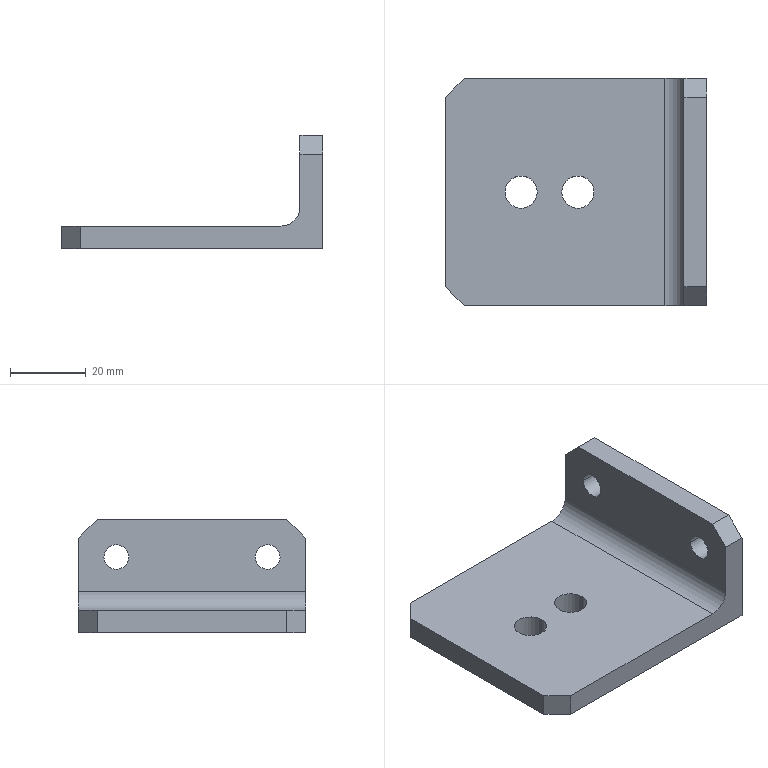Part | SolidWorks | features ICE 3, Chamfer 1, Extrusion 1, Fillet 1 | 1 solid | 21 faces | box 69 x 60 x 30 mm | volume 32423 mm3 | plane 12 | cylinder 9 | commonest cylinder face diameters 6.5 x4 8.5 x4 10 x1
STEP:
#1=CARTESIAN_POINT('',(34.5,23.25,17.));
#2=VERTEX_POINT('',#1);
#3=CARTESIAN_POINT('',(34.5,16.75,17.));
#4=VERTEX_POINT('',#3);
#5=CARTESIAN_POINT('',(34.5,20.,17.));
#6=DIRECTION('',(-1.,0.,0.));
#7=DIRECTION('',(0.,-1.,0.));
#8=AXIS2_PLACEMENT_3D('',#5,#6,#7);
#9=CIRCLE('',#8,3.25);
#10=EDGE_CURVE('',#2,#4,#9,.T.);
#11=ORIENTED_EDGE('',*,*,#10,.F.);
#12=CARTESIAN_POINT('',(28.5,23.25,17.));
#13=VERTEX_POINT('',#12);
#14=CARTESIAN_POINT('',(34.5,23.25,17.));
#15=DIRECTION('',(-1.,0.,0.));
#16=VECTOR('',#15,1000.);
#17=LINE('',#14,#16);
#18=EDGE_CURVE('',#2,#13,#17,.T.);
#19=ORIENTED_EDGE('',*,*,#18,.T.);
#20=CARTESIAN_POINT('',(28.5,16.75,17.));
#21=VERTEX_POINT('',#20);
#22=CARTESIAN_POINT('',(28.5,20.,17.));
#23=DIRECTION('',(-1.,0.,0.));
#24=DIRECTION('',(0.,-1.,0.));
#25=AXIS2_PLACEMENT_3D('',#22,#23,#24);
#26=CIRCLE('',#25,3.25);
#27=EDGE_CURVE('',#13,#21,#26,.T.);
#28=ORIENTED_EDGE('',*,*,#27,.T.);
#29=CARTESIAN_POINT('',(34.5,16.75,17.));
#30=DIRECTION('',(-1.,0.,0.));
#31=VECTOR('',#30,1000.);
#32=LINE('',#29,#31);
#33=EDGE_CURVE('',#4,#21,#32,.T.);
#34=ORIENTED_EDGE('',*,*,#33,.F.);
#35=EDGE_LOOP('',(#11,#19,#28,#34));
#36=FACE_OUTER_BOUND('',#35,.T.);
#37=CARTESIAN_POINT('',(34.5,20.,17.));
#38=DIRECTION('',(-1.,0.,0.));
#39=DIRECTION('',(0.,-1.,0.));
#40=AXIS2_PLACEMENT_3D('',#37,#38,#39);
#41=CYLINDRICAL_SURFACE('',#40,3.25);
#42=ADVANCED_FACE('',(#36),#41,.F.);
#43=CARTESIAN_POINT('',(34.5,-16.75,17.));
#44=VERTEX_POINT('',#43);
#45=CARTESIAN_POINT('',(34.5,-23.25,17.));
#46=VERTEX_POINT('',#45);
#47=CARTESIAN_POINT('',(34.5,-20.,17.));
#48=DIRECTION('',(-1.,0.,0.));
#49=DIRECTION('',(0.,-1.,0.));
#50=AXIS2_PLACEMENT_3D('',#47,#48,#49);
#51=CIRCLE('',#50,3.25);
#52=EDGE_CURVE('',#44,#46,#51,.T.);
#53=ORIENTED_EDGE('',*,*,#52,.F.);
#54=CARTESIAN_POINT('',(28.5,-16.75,17.));
#55=VERTEX_POINT('',#54);
#56=CARTESIAN_POINT('',(34.5,-16.75,17.));
#57=DIRECTION('',(-1.,0.,0.));
#58=VECTOR('',#57,1000.);
#59=LINE('',#56,#58);
#60=EDGE_CURVE('',#44,#55,#59,.T.);
#61=ORIENTED_EDGE('',*,*,#60,.T.);
#62=CARTESIAN_POINT('',(28.5,-23.25,17.));
#63=VERTEX_POINT('',#62);
#64=CARTESIAN_POINT('',(28.5,-20.,17.));
#65=DIRECTION('',(-1.,0.,0.));
#66=DIRECTION('',(0.,-1.,0.));
#67=AXIS2_PLACEMENT_3D('',#64,#65,#66);
#68=CIRCLE('',#67,3.25);
#69=EDGE_CURVE('',#55,#63,#68,.T.);
#70=ORIENTED_EDGE('',*,*,#69,.T.);
#71=CARTESIAN_POINT('',(34.5,-23.25,17.));
#72=DIRECTION('',(-1.,0.,0.));
#73=VECTOR('',#72,1000.);
#74=LINE('',#71,#73);
#75=EDGE_CURVE('',#46,#63,#74,.T.);
#76=ORIENTED_EDGE('',*,*,#75,.F.);
#77=EDGE_LOOP('',(#53,#61,#70,#76));
#78=FACE_OUTER_BOUND('',#77,.T.);
#79=CARTESIAN_POINT('',(34.5,-20.,17.));
#80=DIRECTION('',(-1.,0.,0.));
#81=DIRECTION('',(0.,-1.,0.));
#82=AXIS2_PLACEMENT_3D('',#79,#80,#81);
#83=CYLINDRICAL_SURFACE('',#82,3.25);
#84=ADVANCED_FACE('',(#78),#83,.F.);
#85=CARTESIAN_POINT('',(-18.75,0.,-3.));
#86=VERTEX_POINT('',#85);
#87=CARTESIAN_POINT('',(-10.25,0.,-3.));
#88=VERTEX_POINT('',#87);
#89=CARTESIAN_POINT('',(-14.5,0.,-3.));
#90=DIRECTION('',(0.,0.,1.));
#91=DIRECTION('',(1.,0.,0.));
#92=AXIS2_PLACEMENT_3D('',#89,#90,#91);
#93=CIRCLE('',#92,4.25);
#94=EDGE_CURVE('',#86,#88,#93,.T.);
#95=ORIENTED_EDGE('',*,*,#94,.F.);
#96=CARTESIAN_POINT('',(-18.75,0.,3.));
#97=VERTEX_POINT('',#96);
#98=CARTESIAN_POINT('',(-18.75,0.,-3.));
#99=DIRECTION('',(0.,0.,1.));
#100=VECTOR('',#99,1000.);
#101=LINE('',#98,#100);
#102=EDGE_CURVE('',#86,#97,#101,.T.);
#103=ORIENTED_EDGE('',*,*,#102,.T.);
#104=CARTESIAN_POINT('',(-10.25,0.,3.));
#105=VERTEX_POINT('',#104);
#106=CARTESIAN_POINT('',(-14.5,0.,3.));
#107=DIRECTION('',(0.,0.,1.));
#108=DIRECTION('',(1.,0.,0.));
#109=AXIS2_PLACEMENT_3D('',#106,#107,#108);
#110=CIRCLE('',#109,4.25);
#111=EDGE_CURVE('',#97,#105,#110,.T.);
#112=ORIENTED_EDGE('',*,*,#111,.T.);
#113=CARTESIAN_POINT('',(-10.25,0.,-3.));
#114=DIRECTION('',(0.,0.,1.));
#115=VECTOR('',#114,1000.);
#116=LINE('',#113,#115);
#117=EDGE_CURVE('',#88,#105,#116,.T.);
#118=ORIENTED_EDGE('',*,*,#117,.F.);
#119=EDGE_LOOP('',(#95,#103,#112,#118));
#120=FACE_OUTER_BOUND('',#119,.T.);
#121=CARTESIAN_POINT('',(-14.5,0.,-3.));
#122=DIRECTION('',(0.,0.,1.));
#123=DIRECTION('',(1.,0.,0.));
#124=AXIS2_PLACEMENT_3D('',#121,#122,#123);
#125=CYLINDRICAL_SURFACE('',#124,4.25);
#126=ADVANCED_FACE('',(#120),#125,.F.);
#127=CARTESIAN_POINT('',(-3.75,0.,-3.));
#128=VERTEX_POINT('',#127);
#129=CARTESIAN_POINT('',(4.75,0.,-3.));
#130=VERTEX_POINT('',#129);
#131=CARTESIAN_POINT('',(0.5,0.,-3.));
#132=DIRECTION('',(0.,0.,1.));
#133=DIRECTION('',(1.,0.,0.));
#134=AXIS2_PLACEMENT_3D('',#131,#132,#133);
#135=CIRCLE('',#134,4.25);
#136=EDGE_CURVE('',#128,#130,#135,.T.);
#137=ORIENTED_EDGE('',*,*,#136,.F.);
#138=CARTESIAN_POINT('',(-3.75,0.,3.));
#139=VERTEX_POINT('',#138);
#140=CARTESIAN_POINT('',(-3.75,0.,-3.));
#141=DIRECTION('',(0.,0.,1.));
#142=VECTOR('',#141,1000.);
#143=LINE('',#140,#142);
#144=EDGE_CURVE('',#128,#139,#143,.T.);
#145=ORIENTED_EDGE('',*,*,#144,.T.);
#146=CARTESIAN_POINT('',(4.75,0.,3.));
#147=VERTEX_POINT('',#146);
#148=CARTESIAN_POINT('',(0.5,0.,3.));
#149=DIRECTION('',(0.,0.,1.));
#150=DIRECTION('',(1.,0.,0.));
#151=AXIS2_PLACEMENT_3D('',#148,#149,#150);
#152=CIRCLE('',#151,4.25);
#153=EDGE_CURVE('',#139,#147,#152,.T.);
#154=ORIENTED_EDGE('',*,*,#153,.T.);
#155=CARTESIAN_POINT('',(4.75,0.,-3.));
#156=DIRECTION('',(0.,0.,1.));
#157=VECTOR('',#156,1000.);
#158=LINE('',#155,#157);
#159=EDGE_CURVE('',#130,#147,#158,.T.);
#160=ORIENTED_EDGE('',*,*,#159,.F.);
#161=EDGE_LOOP('',(#137,#145,#154,#160));
#162=FACE_OUTER_BOUND('',#161,.T.);
#163=CARTESIAN_POINT('',(0.5,0.,-3.));
#164=DIRECTION('',(0.,0.,1.));
#165=DIRECTION('',(1.,0.,0.));
#166=AXIS2_PLACEMENT_3D('',#163,#164,#165);
#167=CYLINDRICAL_SURFACE('',#166,4.25);
#168=ADVANCED_FACE('',(#162),#167,.F.);
#169=CARTESIAN_POINT('',(-34.5,25.,3.));
#170=VERTEX_POINT('',#169);
#171=CARTESIAN_POINT('',(-34.5,-25.,3.));
#172=VERTEX_POINT('',#171);
#173=CARTESIAN_POINT('',(-34.5,-30.,3.));
#174=DIRECTION('',(0.,-1.,0.));
#175=VECTOR('',#174,1000.);
#176=LINE('',#173,#175);
#177=EDGE_CURVE('',#170,#172,#176,.T.);
#178=ORIENTED_EDGE('',*,*,#177,.F.);
#179=CARTESIAN_POINT('',(-34.5,25.,-3.));
#180=VERTEX_POINT('',#179);
#181=CARTESIAN_POINT('',(-34.5,25.,3.));
#182=DIRECTION('',(0.,0.,-1.));
#183=VECTOR('',#182,1000.);
#184=LINE('',#181,#183);
#185=EDGE_CURVE('',#170,#180,#184,.T.);
#186=ORIENTED_EDGE('',*,*,#185,.T.);
#187=CARTESIAN_POINT('',(-34.5,-25.,-3.));
#188=VERTEX_POINT('',#187);
#189=CARTESIAN_POINT('',(-34.5,-30.,-3.));
#190=DIRECTION('',(0.,-1.,0.));
#191=VECTOR('',#190,1000.);
#192=LINE('',#189,#191);
#193=EDGE_CURVE('',#180,#188,#192,.T.);
#194=ORIENTED_EDGE('',*,*,#193,.T.);
#195=CARTESIAN_POINT('',(-34.5,-25.,3.));
#196=DIRECTION('',(0.,0.,1.));
#197=VECTOR('',#196,1000.);
#198=LINE('',#195,#197);
#199=EDGE_CURVE('',#188,#172,#198,.T.);
#200=ORIENTED_EDGE('',*,*,#199,.T.);
#201=EDGE_LOOP('',(#178,#186,#194,#200));
#202=FACE_OUTER_BOUND('',#201,.T.);
#203=CARTESIAN_POINT('',(-34.5,-30.,3.));
#204=DIRECTION('',(1.,0.,0.));
#205=DIRECTION('',(0.,0.,-1.));
#206=AXIS2_PLACEMENT_3D('',#203,#204,#205);
#207=PLANE('',#206);
#208=ADVANCED_FACE('',(#202),#207,.F.);
#209=CARTESIAN_POINT('',(-29.5,-30.,3.));
#210=VERTEX_POINT('',#209);
#211=CARTESIAN_POINT('',(23.5,-30.,3.));
#212=VERTEX_POINT('',#211);
#213=CARTESIAN_POINT('',(34.5,-30.,3.));
#214=DIRECTION('',(1.,0.,0.));
#215=VECTOR('',#214,1000.);
#216=LINE('',#213,#215);
#217=EDGE_CURVE('',#210,#212,#216,.T.);
#218=ORIENTED_EDGE('',*,*,#217,.F.);
#219=CARTESIAN_POINT('',(-29.5,-30.,-3.));
#220=VERTEX_POINT('',#219);
#221=CARTESIAN_POINT('',(-29.5,-30.,3.));
#222=DIRECTION('',(0.,0.,-1.));
#223=VECTOR('',#222,1000.);
#224=LINE('',#221,#223);
#225=EDGE_CURVE('',#210,#220,#224,.T.);
#226=ORIENTED_EDGE('',*,*,#225,.T.);
#227=CARTESIAN_POINT('',(34.5,-30.,-3.));
#228=VERTEX_POINT('',#227);
#229=CARTESIAN_POINT('',(34.5,-30.,-3.));
#230=DIRECTION('',(1.,0.,0.));
#231=VECTOR('',#230,1000.);
#232=LINE('',#229,#231);
#233=EDGE_CURVE('',#220,#228,#232,.T.);
#234=ORIENTED_EDGE('',*,*,#233,.T.);
#235=CARTESIAN_POINT('',(34.5,-30.,22.));
#236=VERTEX_POINT('',#235);
#237=CARTESIAN_POINT('',(34.5,-30.,3.));
#238=DIRECTION('',(0.,0.,-1.));
#239=VECTOR('',#238,1000.);
#240=LINE('',#237,#239);
#241=EDGE_CURVE('',#236,#228,#240,.T.);
#242=ORIENTED_EDGE('',*,*,#241,.F.);
#243=CARTESIAN_POINT('',(28.5,-30.,22.));
#244=VERTEX_POINT('',#243);
#245=CARTESIAN_POINT('',(34.5,-30.,22.));
#246=DIRECTION('',(-1.,0.,0.));
#247=VECTOR('',#246,1000.);
#248=LINE('',#245,#247);
#249=EDGE_CURVE('',#236,#244,#248,.T.);
#250=ORIENTED_EDGE('',*,*,#249,.T.);
#251=CARTESIAN_POINT('',(28.5,-30.,8.));
#252=VERTEX_POINT('',#251);
#253=CARTESIAN_POINT('',(28.5,-30.,27.));
#254=DIRECTION('',(0.,0.,-1.));
#255=VECTOR('',#254,1000.);
#256=LINE('',#253,#255);
#257=EDGE_CURVE('',#244,#252,#256,.T.);
#258=ORIENTED_EDGE('',*,*,#257,.T.);
#259=CARTESIAN_POINT('',(23.5,-30.,8.));
#260=DIRECTION('',(0.,1.,0.));
#261=DIRECTION('',(-1.,0.,0.));
#262=AXIS2_PLACEMENT_3D('',#259,#260,#261);
#263=CIRCLE('',#262,5.);
#264=EDGE_CURVE('',#252,#212,#263,.T.);
#265=ORIENTED_EDGE('',*,*,#264,.T.);
#266=EDGE_LOOP('',(#218,#226,#234,#242,#250,#258,#265));
#267=FACE_OUTER_BOUND('',#266,.T.);
#268=CARTESIAN_POINT('',(34.5,-30.,3.));
#269=DIRECTION('',(0.,1.,0.));
#270=DIRECTION('',(-1.,0.,0.));
#271=AXIS2_PLACEMENT_3D('',#268,#269,#270);
#272=PLANE('',#271);
#273=ADVANCED_FACE('',(#267),#272,.F.);
#274=CARTESIAN_POINT('',(34.5,20.,17.));
#275=DIRECTION('',(-1.,0.,0.));
#276=DIRECTION('',(0.,-1.,0.));
#277=AXIS2_PLACEMENT_3D('',#274,#275,#276);
#278=CIRCLE('',#277,3.25);
#279=EDGE_CURVE('',#4,#2,#278,.T.);
#280=ORIENTED_EDGE('',*,*,#279,.T.);
#281=ORIENTED_EDGE('',*,*,#10,.T.);
#282=EDGE_LOOP('',(#280,#281));
#283=FACE_BOUND('',#282,.T.);
#284=CARTESIAN_POINT('',(34.5,-20.,17.));
#285=DIRECTION('',(-1.,0.,0.));
#286=DIRECTION('',(0.,-1.,0.));
#287=AXIS2_PLACEMENT_3D('',#284,#285,#286);
#288=CIRCLE('',#287,3.25);
#289=EDGE_CURVE('',#46,#44,#288,.T.);
#290=ORIENTED_EDGE('',*,*,#289,.T.);
#291=ORIENTED_EDGE('',*,*,#52,.T.);
#292=EDGE_LOOP('',(#290,#291));
#293=FACE_BOUND('',#292,.T.);
#294=CARTESIAN_POINT('',(34.5,30.,22.));
#295=VERTEX_POINT('',#294);
#296=CARTESIAN_POINT('',(34.5,30.,-3.));
#297=VERTEX_POINT('',#296);
#298=CARTESIAN_POINT('',(34.5,30.,3.));
#299=DIRECTION('',(0.,0.,-1.));
#300=VECTOR('',#299,1000.);
#301=LINE('',#298,#300);
#302=EDGE_CURVE('',#295,#297,#301,.T.);
#303=ORIENTED_EDGE('',*,*,#302,.F.);
#304=CARTESIAN_POINT('',(34.5,25.,27.));
#305=VERTEX_POINT('',#304);
#306=CARTESIAN_POINT('',(34.5,25.,27.));
#307=DIRECTION('',(0.,-0.7071,0.7071));
#308=VECTOR('',#307,1000.);
#309=LINE('',#306,#308);
#310=EDGE_CURVE('',#295,#305,#309,.T.);
#311=ORIENTED_EDGE('',*,*,#310,.T.);
#312=CARTESIAN_POINT('',(34.5,-25.,27.));
#313=VERTEX_POINT('',#312);
#314=CARTESIAN_POINT('',(34.5,30.,27.));
#315=DIRECTION('',(0.,1.,0.));
#316=VECTOR('',#315,1000.);
#317=LINE('',#314,#316);
#318=EDGE_CURVE('',#313,#305,#317,.T.);
#319=ORIENTED_EDGE('',*,*,#318,.F.);
#320=CARTESIAN_POINT('',(34.5,-25.,27.));
#321=DIRECTION('',(0.,-0.7071,-0.7071));
#322=VECTOR('',#321,1000.);
#323=LINE('',#320,#322);
#324=EDGE_CURVE('',#313,#236,#323,.T.);
#325=ORIENTED_EDGE('',*,*,#324,.T.);
#326=ORIENTED_EDGE('',*,*,#241,.T.);
#327=CARTESIAN_POINT('',(34.5,-30.,-3.));
#328=DIRECTION('',(0.,1.,0.));
#329=VECTOR('',#328,1000.);
#330=LINE('',#327,#329);
#331=EDGE_CURVE('',#228,#297,#330,.T.);
#332=ORIENTED_EDGE('',*,*,#331,.T.);
#333=EDGE_LOOP('',(#303,#311,#319,#325,#326,#332));
#334=FACE_OUTER_BOUND('',#333,.T.);
#335=CARTESIAN_POINT('',(34.5,-30.,3.));
#336=DIRECTION('',(-1.,0.,0.));
#337=DIRECTION('',(0.,0.,1.));
#338=AXIS2_PLACEMENT_3D('',#335,#336,#337);
#339=PLANE('',#338);
#340=ADVANCED_FACE('',(#283,#293,#334),#339,.F.);
#341=CARTESIAN_POINT('',(-29.5,30.,-3.));
#342=VERTEX_POINT('',#341);
#343=CARTESIAN_POINT('',(34.5,30.,-3.));
#344=DIRECTION('',(-1.,0.,0.));
#345=VECTOR('',#344,1000.);
#346=LINE('',#343,#345);
#347=EDGE_CURVE('',#297,#342,#346,.T.);
#348=ORIENTED_EDGE('',*,*,#347,.T.);
#349=CARTESIAN_POINT('',(-29.5,30.,3.));
#350=VERTEX_POINT('',#349);
#351=CARTESIAN_POINT('',(-29.5,30.,3.));
#352=DIRECTION('',(0.,0.,1.));
#353=VECTOR('',#352,1000.);
#354=LINE('',#351,#353);
#355=EDGE_CURVE('',#342,#350,#354,.T.);
#356=ORIENTED_EDGE('',*,*,#355,.T.);
#357=CARTESIAN_POINT('',(23.5,30.,3.));
#358=VERTEX_POINT('',#357);
#359=CARTESIAN_POINT('',(34.5,30.,3.));
#360=DIRECTION('',(-1.,0.,0.));
#361=VECTOR('',#360,1000.);
#362=LINE('',#359,#361);
#363=EDGE_CURVE('',#358,#350,#362,.T.);
#364=ORIENTED_EDGE('',*,*,#363,.F.);
#365=CARTESIAN_POINT('',(28.5,30.,8.));
#366=VERTEX_POINT('',#365);
#367=CARTESIAN_POINT('',(23.5,30.,8.));
#368=DIRECTION('',(0.,-1.,0.));
#369=DIRECTION('',(1.,0.,0.));
#370=AXIS2_PLACEMENT_3D('',#367,#368,#369);
#371=CIRCLE('',#370,5.);
#372=EDGE_CURVE('',#358,#366,#371,.T.);
#373=ORIENTED_EDGE('',*,*,#372,.T.);
#374=CARTESIAN_POINT('',(28.5,30.,22.));
#375=VERTEX_POINT('',#374);
#376=CARTESIAN_POINT('',(28.5,30.,27.));
#377=DIRECTION('',(0.,0.,-1.));
#378=VECTOR('',#377,1000.);
#379=LINE('',#376,#378);
#380=EDGE_CURVE('',#375,#366,#379,.T.);
#381=ORIENTED_EDGE('',*,*,#380,.F.);
#382=CARTESIAN_POINT('',(34.5,30.,22.));
#383=DIRECTION('',(1.,0.,0.));
#384=VECTOR('',#383,1000.);
#385=LINE('',#382,#384);
#386=EDGE_CURVE('',#375,#295,#385,.T.);
#387=ORIENTED_EDGE('',*,*,#386,.T.);
#388=ORIENTED_EDGE('',*,*,#302,.T.);
#389=EDGE_LOOP('',(#348,#356,#364,#373,#381,#387,#388));
#390=FACE_OUTER_BOUND('',#389,.T.);
#391=CARTESIAN_POINT('',(34.5,30.,3.));
#392=DIRECTION('',(0.,-1.,0.));
#393=DIRECTION('',(1.,0.,0.));
#394=AXIS2_PLACEMENT_3D('',#391,#392,#393);
#395=PLANE('',#394);
#396=ADVANCED_FACE('',(#390),#395,.F.);
#397=CARTESIAN_POINT('',(-14.5,0.,3.));
#398=DIRECTION('',(0.,0.,1.));
#399=DIRECTION('',(1.,0.,0.));
#400=AXIS2_PLACEMENT_3D('',#397,#398,#399);
#401=CIRCLE('',#400,4.25);
#402=EDGE_CURVE('',#105,#97,#401,.T.);
#403=ORIENTED_EDGE('',*,*,#402,.F.);
#404=ORIENTED_EDGE('',*,*,#111,.F.);
#405=EDGE_LOOP('',(#403,#404));
#406=FACE_BOUND('',#405,.T.);
#407=CARTESIAN_POINT('',(0.5,0.,3.));
#408=DIRECTION('',(0.,0.,1.));
#409=DIRECTION('',(1.,0.,0.));
#410=AXIS2_PLACEMENT_3D('',#407,#408,#409);
#411=CIRCLE('',#410,4.25);
#412=EDGE_CURVE('',#147,#139,#411,.T.);
#413=ORIENTED_EDGE('',*,*,#412,.F.);
#414=ORIENTED_EDGE('',*,*,#153,.F.);
#415=EDGE_LOOP('',(#413,#414));
#416=FACE_BOUND('',#415,.T.);
#417=ORIENTED_EDGE('',*,*,#217,.T.);
#418=CARTESIAN_POINT('',(23.5,0.,3.));
#419=DIRECTION('',(0.,1.,0.));
#420=VECTOR('',#419,1000.);
#421=LINE('',#418,#420);
#422=EDGE_CURVE('',#212,#358,#421,.T.);
#423=ORIENTED_EDGE('',*,*,#422,.T.);
#424=ORIENTED_EDGE('',*,*,#363,.T.);
#425=CARTESIAN_POINT('',(-29.75,29.75,3.));
#426=DIRECTION('',(-0.7071,-0.7071,0.));
#427=VECTOR('',#426,1000.);
#428=LINE('',#425,#427);
#429=EDGE_CURVE('',#350,#170,#428,.T.);
#430=ORIENTED_EDGE('',*,*,#429,.T.);
#431=ORIENTED_EDGE('',*,*,#177,.T.);
#432=CARTESIAN_POINT('',(-29.75,-29.75,3.));
#433=DIRECTION('',(0.7071,-0.7071,0.));
#434=VECTOR('',#433,1000.);
#435=LINE('',#432,#434);
#436=EDGE_CURVE('',#172,#210,#435,.T.);
#437=ORIENTED_EDGE('',*,*,#436,.T.);
#438=EDGE_LOOP('',(#417,#423,#424,#430,#431,#437));
#439=FACE_OUTER_BOUND('',#438,.T.);
#440=CARTESIAN_POINT('',(0.,0.,3.));
#441=DIRECTION('',(0.,0.,1.));
#442=DIRECTION('',(1.,0.,0.));
#443=AXIS2_PLACEMENT_3D('',#440,#441,#442);
#444=PLANE('',#443);
#445=ADVANCED_FACE('',(#406,#416,#439),#444,.T.);
#446=CARTESIAN_POINT('',(-14.5,0.,-3.));
#447=DIRECTION('',(0.,0.,1.));
#448=DIRECTION('',(1.,0.,0.));
#449=AXIS2_PLACEMENT_3D('',#446,#447,#448);
#450=CIRCLE('',#449,4.25);
#451=EDGE_CURVE('',#88,#86,#450,.T.);
#452=ORIENTED_EDGE('',*,*,#451,.T.);
#453=ORIENTED_EDGE('',*,*,#94,.T.);
#454=EDGE_LOOP('',(#452,#453));
#455=FACE_BOUND('',#454,.T.);
#456=CARTESIAN_POINT('',(0.5,0.,-3.));
#457=DIRECTION('',(0.,0.,1.));
#458=DIRECTION('',(1.,0.,0.));
#459=AXIS2_PLACEMENT_3D('',#456,#457,#458);
#460=CIRCLE('',#459,4.25);
#461=EDGE_CURVE('',#130,#128,#460,.T.);
#462=ORIENTED_EDGE('',*,*,#461,.T.);
#463=ORIENTED_EDGE('',*,*,#136,.T.);
#464=EDGE_LOOP('',(#462,#463));
#465=FACE_BOUND('',#464,.T.);
#466=ORIENTED_EDGE('',*,*,#193,.F.);
#467=CARTESIAN_POINT('',(-34.5,25.,-3.));
#468=DIRECTION('',(0.7071,0.7071,0.));
#469=VECTOR('',#468,1000.);
#470=LINE('',#467,#469);
#471=EDGE_CURVE('',#180,#342,#470,.T.);
#472=ORIENTED_EDGE('',*,*,#471,.T.);
#473=ORIENTED_EDGE('',*,*,#347,.F.);
#474=ORIENTED_EDGE('',*,*,#331,.F.);
#475=ORIENTED_EDGE('',*,*,#233,.F.);
#476=CARTESIAN_POINT('',(-29.5,-30.,-3.));
#477=DIRECTION('',(-0.7071,0.7071,0.));
#478=VECTOR('',#477,1000.);
#479=LINE('',#476,#478);
#480=EDGE_CURVE('',#220,#188,#479,.T.);
#481=ORIENTED_EDGE('',*,*,#480,.T.);
#482=EDGE_LOOP('',(#466,#472,#473,#474,#475,#481));
#483=FACE_OUTER_BOUND('',#482,.T.);
#484=CARTESIAN_POINT('',(0.,0.,-3.));
#485=DIRECTION('',(0.,0.,1.));
#486=DIRECTION('',(1.,0.,0.));
#487=AXIS2_PLACEMENT_3D('',#484,#485,#486);
#488=PLANE('',#487);
#489=ADVANCED_FACE('',(#455,#465,#483),#488,.F.);
#490=CARTESIAN_POINT('',(28.5,20.,17.));
#491=DIRECTION('',(-1.,0.,0.));
#492=DIRECTION('',(0.,-1.,0.));
#493=AXIS2_PLACEMENT_3D('',#490,#491,#492);
#494=CIRCLE('',#493,3.25);
#495=EDGE_CURVE('',#21,#13,#494,.T.);
#496=ORIENTED_EDGE('',*,*,#495,.F.);
#497=ORIENTED_EDGE('',*,*,#27,.F.);
#498=EDGE_LOOP('',(#496,#497));
#499=FACE_BOUND('',#498,.T.);
#500=CARTESIAN_POINT('',(28.5,-20.,17.));
#501=DIRECTION('',(-1.,0.,0.));
#502=DIRECTION('',(0.,-1.,0.));
#503=AXIS2_PLACEMENT_3D('',#500,#501,#502);
#504=CIRCLE('',#503,3.25);
#505=EDGE_CURVE('',#63,#55,#504,.T.);
#506=ORIENTED_EDGE('',*,*,#505,.F.);
#507=ORIENTED_EDGE('',*,*,#69,.F.);
#508=EDGE_LOOP('',(#506,#507));
#509=FACE_BOUND('',#508,.T.);
#510=ORIENTED_EDGE('',*,*,#380,.T.);
#511=CARTESIAN_POINT('',(28.5,30.,8.));
#512=DIRECTION('',(0.,-1.,0.));
#513=VECTOR('',#512,1000.);
#514=LINE('',#511,#513);
#515=EDGE_CURVE('',#366,#252,#514,.T.);
#516=ORIENTED_EDGE('',*,*,#515,.T.);
#517=ORIENTED_EDGE('',*,*,#257,.F.);
#518=CARTESIAN_POINT('',(28.5,-25.,27.));
#519=VERTEX_POINT('',#518);
#520=CARTESIAN_POINT('',(28.5,-25.,27.));
#521=DIRECTION('',(0.,0.7071,0.7071));
#522=VECTOR('',#521,1000.);
#523=LINE('',#520,#522);
#524=EDGE_CURVE('',#244,#519,#523,.T.);
#525=ORIENTED_EDGE('',*,*,#524,.T.);
#526=CARTESIAN_POINT('',(28.5,25.,27.));
#527=VERTEX_POINT('',#526);
#528=CARTESIAN_POINT('',(28.5,30.,27.));
#529=DIRECTION('',(0.,-1.,0.));
#530=VECTOR('',#529,1000.);
#531=LINE('',#528,#530);
#532=EDGE_CURVE('',#527,#519,#531,.T.);
#533=ORIENTED_EDGE('',*,*,#532,.F.);
#534=CARTESIAN_POINT('',(28.5,25.,27.));
#535=DIRECTION('',(0.,0.7071,-0.7071));
#536=VECTOR('',#535,1000.);
#537=LINE('',#534,#536);
#538=EDGE_CURVE('',#527,#375,#537,.T.);
#539=ORIENTED_EDGE('',*,*,#538,.T.);
#540=EDGE_LOOP('',(#510,#516,#517,#525,#533,#539));
#541=FACE_OUTER_BOUND('',#540,.T.);
#542=CARTESIAN_POINT('',(28.5,30.,27.));
#543=DIRECTION('',(1.,0.,0.));
#544=DIRECTION('',(0.,1.,0.));
#545=AXIS2_PLACEMENT_3D('',#542,#543,#544);
#546=PLANE('',#545);
#547=ADVANCED_FACE('',(#499,#509,#541),#546,.F.);
#548=ORIENTED_EDGE('',*,*,#318,.T.);
#549=CARTESIAN_POINT('',(0.,25.,27.));
#550=DIRECTION('',(-1.,0.,0.));
#551=VECTOR('',#550,1000.);
#552=LINE('',#549,#551);
#553=EDGE_CURVE('',#305,#527,#552,.T.);
#554=ORIENTED_EDGE('',*,*,#553,.T.);
#555=ORIENTED_EDGE('',*,*,#532,.T.);
#556=CARTESIAN_POINT('',(0.,-25.,27.));
#557=DIRECTION('',(1.,0.,0.));
#558=VECTOR('',#557,1000.);
#559=LINE('',#556,#558);
#560=EDGE_CURVE('',#519,#313,#559,.T.);
#561=ORIENTED_EDGE('',*,*,#560,.T.);
#562=EDGE_LOOP('',(#548,#554,#555,#561));
#563=FACE_OUTER_BOUND('',#562,.T.);
#564=CARTESIAN_POINT('',(0.,0.,27.));
#565=DIRECTION('',(0.,0.,-1.));
#566=DIRECTION('',(-1.,0.,0.));
#567=AXIS2_PLACEMENT_3D('',#564,#565,#566);
#568=PLANE('',#567);
#569=ADVANCED_FACE('',(#563),#568,.F.);
#570=ORIENTED_EDGE('',*,*,#429,.F.);
#571=ORIENTED_EDGE('',*,*,#355,.F.);
#572=ORIENTED_EDGE('',*,*,#471,.F.);
#573=ORIENTED_EDGE('',*,*,#185,.F.);
#574=EDGE_LOOP('',(#570,#571,#572,#573));
#575=FACE_OUTER_BOUND('',#574,.T.);
#576=CARTESIAN_POINT('',(-34.5,25.,3.));
#577=DIRECTION('',(0.7071,-0.7071,0.));
#578=DIRECTION('',(0.,0.,-1.));
#579=AXIS2_PLACEMENT_3D('',#576,#577,#578);
#580=PLANE('',#579);
#581=ADVANCED_FACE('',(#575),#580,.F.);
#582=ORIENTED_EDGE('',*,*,#436,.F.);
#583=ORIENTED_EDGE('',*,*,#199,.F.);
#584=ORIENTED_EDGE('',*,*,#480,.F.);
#585=ORIENTED_EDGE('',*,*,#225,.F.);
#586=EDGE_LOOP('',(#582,#583,#584,#585));
#587=FACE_OUTER_BOUND('',#586,.T.);
#588=CARTESIAN_POINT('',(-29.5,-30.,3.));
#589=DIRECTION('',(0.7071,0.7071,0.));
#590=DIRECTION('',(0.,0.,-1.));
#591=AXIS2_PLACEMENT_3D('',#588,#589,#590);
#592=PLANE('',#591);
#593=ADVANCED_FACE('',(#587),#592,.F.);
#594=ORIENTED_EDGE('',*,*,#310,.F.);
#595=ORIENTED_EDGE('',*,*,#386,.F.);
#596=ORIENTED_EDGE('',*,*,#538,.F.);
#597=ORIENTED_EDGE('',*,*,#553,.F.);
#598=EDGE_LOOP('',(#594,#595,#596,#597));
#599=FACE_OUTER_BOUND('',#598,.T.);
#600=CARTESIAN_POINT('',(0.,25.,27.));
#601=DIRECTION('',(0.,-0.7071,-0.7071));
#602=DIRECTION('',(-1.,0.,0.));
#603=AXIS2_PLACEMENT_3D('',#600,#601,#602);
#604=PLANE('',#603);
#605=ADVANCED_FACE('',(#599),#604,.F.);
#606=ORIENTED_EDGE('',*,*,#524,.F.);
#607=ORIENTED_EDGE('',*,*,#249,.F.);
#608=ORIENTED_EDGE('',*,*,#324,.F.);
#609=ORIENTED_EDGE('',*,*,#560,.F.);
#610=EDGE_LOOP('',(#606,#607,#608,#609));
#611=FACE_OUTER_BOUND('',#610,.T.);
#612=CARTESIAN_POINT('',(0.,-25.,27.));
#613=DIRECTION('',(0.,0.7071,-0.7071));
#614=DIRECTION('',(1.,0.,0.));
#615=AXIS2_PLACEMENT_3D('',#612,#613,#614);
#616=PLANE('',#615);
#617=ADVANCED_FACE('',(#611),#616,.F.);
#618=ORIENTED_EDGE('',*,*,#144,.F.);
#619=ORIENTED_EDGE('',*,*,#461,.F.);
#620=ORIENTED_EDGE('',*,*,#159,.T.);
#621=ORIENTED_EDGE('',*,*,#412,.T.);
#622=EDGE_LOOP('',(#618,#619,#620,#621));
#623=FACE_OUTER_BOUND('',#622,.T.);
#624=CARTESIAN_POINT('',(0.5,0.,-3.));
#625=DIRECTION('',(0.,0.,1.));
#626=DIRECTION('',(1.,0.,0.));
#627=AXIS2_PLACEMENT_3D('',#624,#625,#626);
#628=CYLINDRICAL_SURFACE('',#627,4.25);
#629=ADVANCED_FACE('',(#623),#628,.F.);
#630=ORIENTED_EDGE('',*,*,#102,.F.);
#631=ORIENTED_EDGE('',*,*,#451,.F.);
#632=ORIENTED_EDGE('',*,*,#117,.T.);
#633=ORIENTED_EDGE('',*,*,#402,.T.);
#634=EDGE_LOOP('',(#630,#631,#632,#633));
#635=FACE_OUTER_BOUND('',#634,.T.);
#636=CARTESIAN_POINT('',(-14.5,0.,-3.));
#637=DIRECTION('',(0.,0.,1.));
#638=DIRECTION('',(1.,0.,0.));
#639=AXIS2_PLACEMENT_3D('',#636,#637,#638);
#640=CYLINDRICAL_SURFACE('',#639,4.25);
#641=ADVANCED_FACE('',(#635),#640,.F.);
#642=ORIENTED_EDGE('',*,*,#372,.F.);
#643=ORIENTED_EDGE('',*,*,#422,.F.);
#644=ORIENTED_EDGE('',*,*,#264,.F.);
#645=ORIENTED_EDGE('',*,*,#515,.F.);
#646=EDGE_LOOP('',(#642,#643,#644,#645));
#647=FACE_OUTER_BOUND('',#646,.T.);
#648=CARTESIAN_POINT('',(23.5,30.,8.));
#649=DIRECTION('',(0.,-1.,0.));
#650=DIRECTION('',(1.,0.,0.));
#651=AXIS2_PLACEMENT_3D('',#648,#649,#650);
#652=CYLINDRICAL_SURFACE('',#651,5.);
#653=ADVANCED_FACE('',(#647),#652,.F.);
#654=ORIENTED_EDGE('',*,*,#60,.F.);
#655=ORIENTED_EDGE('',*,*,#289,.F.);
#656=ORIENTED_EDGE('',*,*,#75,.T.);
#657=ORIENTED_EDGE('',*,*,#505,.T.);
#658=EDGE_LOOP('',(#654,#655,#656,#657));
#659=FACE_OUTER_BOUND('',#658,.T.);
#660=CARTESIAN_POINT('',(34.5,-20.,17.));
#661=DIRECTION('',(-1.,0.,0.));
#662=DIRECTION('',(0.,-1.,0.));
#663=AXIS2_PLACEMENT_3D('',#660,#661,#662);
#664=CYLINDRICAL_SURFACE('',#663,3.25);
#665=ADVANCED_FACE('',(#659),#664,.F.);
#666=ORIENTED_EDGE('',*,*,#18,.F.);
#667=ORIENTED_EDGE('',*,*,#279,.F.);
#668=ORIENTED_EDGE('',*,*,#33,.T.);
#669=ORIENTED_EDGE('',*,*,#495,.T.);
#670=EDGE_LOOP('',(#666,#667,#668,#669));
#671=FACE_OUTER_BOUND('',#670,.T.);
#672=CARTESIAN_POINT('',(34.5,20.,17.));
#673=DIRECTION('',(-1.,0.,0.));
#674=DIRECTION('',(0.,-1.,0.));
#675=AXIS2_PLACEMENT_3D('',#672,#673,#674);
#676=CYLINDRICAL_SURFACE('',#675,3.25);
#677=ADVANCED_FACE('',(#671),#676,.F.);
#678=CLOSED_SHELL('',(#42,#84,#126,#168,#208,#273,#340,#396,#445,#489,#547,#569,#581,#593,#605,#617,#629,#641,#653,#665,#677));
#679=MANIFOLD_SOLID_BREP('',#678);
#680=CARTESIAN_POINT('',(0.,0.,0.));
#681=DIRECTION('',(0.,0.,1.));
#682=DIRECTION('',(1.,0.,0.));
#683=AXIS2_PLACEMENT_3D('',#680,#681,#682);
#684=(LENGTH_UNIT()NAMED_UNIT(*)SI_UNIT(.MILLI.,.METRE.));
#685=UNCERTAINTY_MEASURE_WITH_UNIT(LENGTH_MEASURE(0.00001),#684,'','');
#686=(NAMED_UNIT(*)PLANE_ANGLE_UNIT()SI_UNIT($,.RADIAN.));
#687=(NAMED_UNIT(*)SI_UNIT($,.STERADIAN.)SOLID_ANGLE_UNIT());
#688=(GEOMETRIC_REPRESENTATION_CONTEXT(3)GLOBAL_UNCERTAINTY_ASSIGNED_CONTEXT((#685))GLOBAL_UNIT_ASSIGNED_CONTEXT((#684,#686,#687))REPRESENTATION_CONTEXT('',''));
#689=ADVANCED_BREP_SHAPE_REPRESENTATION('',(#679,#683),#688);